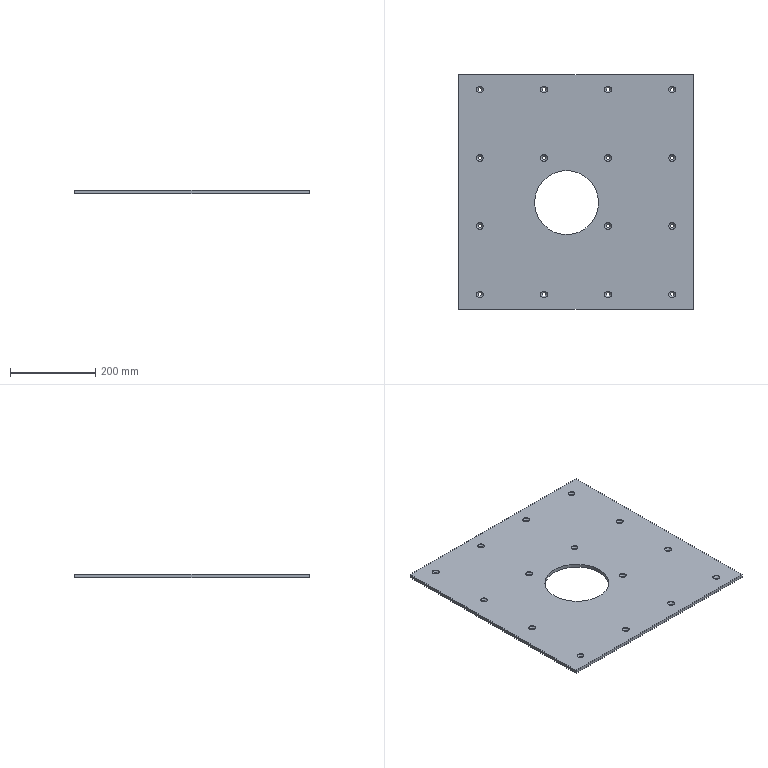Part | STEP file | 车灯-后视镜_id582_x_t | 1 solid | 52 faces | box 550 x 550 x 8 mm | volume 2264649 mm3 | cylinder 31 | cone 15 | plane 6 | commonest cylinder face diameters 8.5 x15 16 x15 150 x1
STEP:
#1=CARTESIAN_POINT('',(275.,-275.,225.5));
#2=VERTEX_POINT('',#1);
#3=CARTESIAN_POINT('',(-275.,-275.,225.5));
#4=VERTEX_POINT('',#3);
#5=CARTESIAN_POINT('',(275.,-275.,225.5));
#6=DIRECTION('',(-1.,0.,0.));
#7=VECTOR('',#6,1.);
#8=LINE('',#5,#7);
#9=EDGE_CURVE('',#2,#4,#8,.T.);
#10=ORIENTED_EDGE('',*,*,#9,.F.);
#11=CARTESIAN_POINT('',(275.,-275.,233.5));
#12=VERTEX_POINT('',#11);
#13=CARTESIAN_POINT('',(275.,-275.,233.5));
#14=DIRECTION('',(0.,0.,-1.));
#15=VECTOR('',#14,1.);
#16=LINE('',#13,#15);
#17=EDGE_CURVE('',#12,#2,#16,.T.);
#18=ORIENTED_EDGE('',*,*,#17,.F.);
#19=CARTESIAN_POINT('',(-275.,-275.,233.5));
#20=VERTEX_POINT('',#19);
#21=CARTESIAN_POINT('',(275.,-275.,233.5));
#22=DIRECTION('',(-1.,0.,0.));
#23=VECTOR('',#22,1.);
#24=LINE('',#21,#23);
#25=EDGE_CURVE('',#12,#20,#24,.T.);
#26=ORIENTED_EDGE('',*,*,#25,.T.);
#27=CARTESIAN_POINT('',(-275.,-275.,233.5));
#28=DIRECTION('',(0.,0.,-1.));
#29=VECTOR('',#28,1.);
#30=LINE('',#27,#29);
#31=EDGE_CURVE('',#20,#4,#30,.T.);
#32=ORIENTED_EDGE('',*,*,#31,.T.);
#33=EDGE_LOOP('',(#10,#18,#26,#32));
#34=FACE_OUTER_BOUND('',#33,.T.);
#35=CARTESIAN_POINT('',(275.,-275.,233.5));
#36=DIRECTION('',(0.,-1.,0.));
#37=DIRECTION('',(0.,0.,-1.));
#38=AXIS2_PLACEMENT_3D('',#35,#36,#37);
#39=PLANE('',#38);
#40=ADVANCED_FACE('',(#34),#39,.T.);
#41=CARTESIAN_POINT('',(-275.,275.,225.5));
#42=VERTEX_POINT('',#41);
#43=CARTESIAN_POINT('',(-275.,-275.,225.5));
#44=DIRECTION('',(0.,1.,0.));
#45=VECTOR('',#44,1.);
#46=LINE('',#43,#45);
#47=EDGE_CURVE('',#4,#42,#46,.T.);
#48=ORIENTED_EDGE('',*,*,#47,.F.);
#49=ORIENTED_EDGE('',*,*,#31,.F.);
#50=CARTESIAN_POINT('',(-275.,275.,233.5));
#51=VERTEX_POINT('',#50);
#52=CARTESIAN_POINT('',(-275.,-275.,233.5));
#53=DIRECTION('',(0.,1.,0.));
#54=VECTOR('',#53,1.);
#55=LINE('',#52,#54);
#56=EDGE_CURVE('',#20,#51,#55,.T.);
#57=ORIENTED_EDGE('',*,*,#56,.T.);
#58=CARTESIAN_POINT('',(-275.,275.,233.5));
#59=DIRECTION('',(0.,0.,-1.));
#60=VECTOR('',#59,1.);
#61=LINE('',#58,#60);
#62=EDGE_CURVE('',#51,#42,#61,.T.);
#63=ORIENTED_EDGE('',*,*,#62,.T.);
#64=EDGE_LOOP('',(#48,#49,#57,#63));
#65=FACE_OUTER_BOUND('',#64,.T.);
#66=CARTESIAN_POINT('',(-275.,-275.,233.5));
#67=DIRECTION('',(-1.,0.,0.));
#68=DIRECTION('',(0.,0.,1.));
#69=AXIS2_PLACEMENT_3D('',#66,#67,#68);
#70=PLANE('',#69);
#71=ADVANCED_FACE('',(#65),#70,.T.);
#72=CARTESIAN_POINT('',(275.,275.,225.5));
#73=VERTEX_POINT('',#72);
#74=CARTESIAN_POINT('',(-275.,275.,225.5));
#75=DIRECTION('',(1.,0.,0.));
#76=VECTOR('',#75,1.);
#77=LINE('',#74,#76);
#78=EDGE_CURVE('',#42,#73,#77,.T.);
#79=ORIENTED_EDGE('',*,*,#78,.F.);
#80=ORIENTED_EDGE('',*,*,#62,.F.);
#81=CARTESIAN_POINT('',(275.,275.,233.5));
#82=VERTEX_POINT('',#81);
#83=CARTESIAN_POINT('',(-275.,275.,233.5));
#84=DIRECTION('',(1.,0.,0.));
#85=VECTOR('',#84,1.);
#86=LINE('',#83,#85);
#87=EDGE_CURVE('',#51,#82,#86,.T.);
#88=ORIENTED_EDGE('',*,*,#87,.T.);
#89=CARTESIAN_POINT('',(275.,275.,233.5));
#90=DIRECTION('',(0.,0.,-1.));
#91=VECTOR('',#90,1.);
#92=LINE('',#89,#91);
#93=EDGE_CURVE('',#82,#73,#92,.T.);
#94=ORIENTED_EDGE('',*,*,#93,.T.);
#95=EDGE_LOOP('',(#79,#80,#88,#94));
#96=FACE_OUTER_BOUND('',#95,.T.);
#97=CARTESIAN_POINT('',(-275.,275.,233.5));
#98=DIRECTION('',(0.,1.,0.));
#99=DIRECTION('',(0.,0.,1.));
#100=AXIS2_PLACEMENT_3D('',#97,#98,#99);
#101=PLANE('',#100);
#102=ADVANCED_FACE('',(#96),#101,.T.);
#103=CARTESIAN_POINT('',(275.,275.,225.5));
#104=DIRECTION('',(0.,-1.,0.));
#105=VECTOR('',#104,1.);
#106=LINE('',#103,#105);
#107=EDGE_CURVE('',#73,#2,#106,.T.);
#108=ORIENTED_EDGE('',*,*,#107,.F.);
#109=ORIENTED_EDGE('',*,*,#93,.F.);
#110=CARTESIAN_POINT('',(275.,275.,233.5));
#111=DIRECTION('',(0.,-1.,0.));
#112=VECTOR('',#111,1.);
#113=LINE('',#110,#112);
#114=EDGE_CURVE('',#82,#12,#113,.T.);
#115=ORIENTED_EDGE('',*,*,#114,.T.);
#116=ORIENTED_EDGE('',*,*,#17,.T.);
#117=EDGE_LOOP('',(#108,#109,#115,#116));
#118=FACE_OUTER_BOUND('',#117,.T.);
#119=CARTESIAN_POINT('',(275.,275.,233.5));
#120=DIRECTION('',(1.,0.,0.));
#121=DIRECTION('',(0.,0.,-1.));
#122=AXIS2_PLACEMENT_3D('',#119,#120,#121);
#123=PLANE('',#122);
#124=ADVANCED_FACE('',(#118),#123,.T.);
#125=CARTESIAN_POINT('',(-233.,240.,233.5));
#126=VERTEX_POINT('',#125);
#127=CARTESIAN_POINT('',(-225.,240.,233.5));
#128=DIRECTION('',(0.,0.,-1.));
#129=DIRECTION('',(-1.,0.,0.));
#130=AXIS2_PLACEMENT_3D('',#127,#128,#129);
#131=CIRCLE('',#130,8.);
#132=EDGE_CURVE('',#126,#126,#131,.T.);
#133=ORIENTED_EDGE('',*,*,#132,.T.);
#134=EDGE_LOOP('',(#133));
#135=FACE_BOUND('',#134,.T.);
#136=CARTESIAN_POINT('',(-233.,-240.,233.5));
#137=VERTEX_POINT('',#136);
#138=CARTESIAN_POINT('',(-225.,-240.,233.5));
#139=DIRECTION('',(0.,0.,-1.));
#140=DIRECTION('',(-1.,0.,0.));
#141=AXIS2_PLACEMENT_3D('',#138,#139,#140);
#142=CIRCLE('',#141,8.);
#143=EDGE_CURVE('',#137,#137,#142,.T.);
#144=ORIENTED_EDGE('',*,*,#143,.T.);
#145=EDGE_LOOP('',(#144));
#146=FACE_BOUND('',#145,.T.);
#147=CARTESIAN_POINT('',(-83.,80.,233.5));
#148=VERTEX_POINT('',#147);
#149=CARTESIAN_POINT('',(-75.,80.,233.5));
#150=DIRECTION('',(0.,0.,-1.));
#151=DIRECTION('',(-1.,0.,0.));
#152=AXIS2_PLACEMENT_3D('',#149,#150,#151);
#153=CIRCLE('',#152,8.);
#154=EDGE_CURVE('',#148,#148,#153,.T.);
#155=ORIENTED_EDGE('',*,*,#154,.T.);
#156=EDGE_LOOP('',(#155));
#157=FACE_BOUND('',#156,.T.);
#158=CARTESIAN_POINT('',(-233.,-80.,233.5));
#159=VERTEX_POINT('',#158);
#160=CARTESIAN_POINT('',(-225.,-80.,233.5));
#161=DIRECTION('',(0.,0.,-1.));
#162=DIRECTION('',(-1.,0.,0.));
#163=AXIS2_PLACEMENT_3D('',#160,#161,#162);
#164=CIRCLE('',#163,8.);
#165=EDGE_CURVE('',#159,#159,#164,.T.);
#166=ORIENTED_EDGE('',*,*,#165,.T.);
#167=EDGE_LOOP('',(#166));
#168=FACE_BOUND('',#167,.T.);
#169=CARTESIAN_POINT('',(-233.,80.,233.5));
#170=VERTEX_POINT('',#169);
#171=CARTESIAN_POINT('',(-225.,80.,233.5));
#172=DIRECTION('',(0.,0.,-1.));
#173=DIRECTION('',(-1.,0.,0.));
#174=AXIS2_PLACEMENT_3D('',#171,#172,#173);
#175=CIRCLE('',#174,8.);
#176=EDGE_CURVE('',#170,#170,#175,.T.);
#177=ORIENTED_EDGE('',*,*,#176,.T.);
#178=EDGE_LOOP('',(#177));
#179=FACE_BOUND('',#178,.T.);
#180=CARTESIAN_POINT('',(-83.,-240.,233.5));
#181=VERTEX_POINT('',#180);
#182=CARTESIAN_POINT('',(-75.,-240.,233.5));
#183=DIRECTION('',(0.,0.,-1.));
#184=DIRECTION('',(-1.,0.,0.));
#185=AXIS2_PLACEMENT_3D('',#182,#183,#184);
#186=CIRCLE('',#185,8.);
#187=EDGE_CURVE('',#181,#181,#186,.T.);
#188=ORIENTED_EDGE('',*,*,#187,.T.);
#189=EDGE_LOOP('',(#188));
#190=FACE_BOUND('',#189,.T.);
#191=CARTESIAN_POINT('',(-83.,240.,233.5));
#192=VERTEX_POINT('',#191);
#193=CARTESIAN_POINT('',(-75.,240.,233.5));
#194=DIRECTION('',(0.,0.,-1.));
#195=DIRECTION('',(-1.,0.,0.));
#196=AXIS2_PLACEMENT_3D('',#193,#194,#195);
#197=CIRCLE('',#196,8.);
#198=EDGE_CURVE('',#192,#192,#197,.T.);
#199=ORIENTED_EDGE('',*,*,#198,.T.);
#200=EDGE_LOOP('',(#199));
#201=FACE_BOUND('',#200,.T.);
#202=CARTESIAN_POINT('',(67.,240.,233.5));
#203=VERTEX_POINT('',#202);
#204=CARTESIAN_POINT('',(75.,240.,233.5));
#205=DIRECTION('',(0.,0.,-1.));
#206=DIRECTION('',(-1.,0.,0.));
#207=AXIS2_PLACEMENT_3D('',#204,#205,#206);
#208=CIRCLE('',#207,8.);
#209=EDGE_CURVE('',#203,#203,#208,.T.);
#210=ORIENTED_EDGE('',*,*,#209,.T.);
#211=EDGE_LOOP('',(#210));
#212=FACE_BOUND('',#211,.T.);
#213=CARTESIAN_POINT('',(217.,80.,233.5));
#214=VERTEX_POINT('',#213);
#215=CARTESIAN_POINT('',(225.,80.,233.5));
#216=DIRECTION('',(0.,0.,-1.));
#217=DIRECTION('',(-1.,0.,0.));
#218=AXIS2_PLACEMENT_3D('',#215,#216,#217);
#219=CIRCLE('',#218,8.);
#220=EDGE_CURVE('',#214,#214,#219,.T.);
#221=ORIENTED_EDGE('',*,*,#220,.T.);
#222=EDGE_LOOP('',(#221));
#223=FACE_BOUND('',#222,.T.);
#224=CARTESIAN_POINT('',(217.,240.,233.5));
#225=VERTEX_POINT('',#224);
#226=CARTESIAN_POINT('',(225.,240.,233.5));
#227=DIRECTION('',(0.,0.,-1.));
#228=DIRECTION('',(-1.,0.,0.));
#229=AXIS2_PLACEMENT_3D('',#226,#227,#228);
#230=CIRCLE('',#229,8.);
#231=EDGE_CURVE('',#225,#225,#230,.T.);
#232=ORIENTED_EDGE('',*,*,#231,.T.);
#233=EDGE_LOOP('',(#232));
#234=FACE_BOUND('',#233,.T.);
#235=CARTESIAN_POINT('',(67.,-240.,233.5));
#236=VERTEX_POINT('',#235);
#237=CARTESIAN_POINT('',(75.,-240.,233.5));
#238=DIRECTION('',(0.,0.,-1.));
#239=DIRECTION('',(-1.,0.,0.));
#240=AXIS2_PLACEMENT_3D('',#237,#238,#239);
#241=CIRCLE('',#240,8.);
#242=EDGE_CURVE('',#236,#236,#241,.T.);
#243=ORIENTED_EDGE('',*,*,#242,.T.);
#244=EDGE_LOOP('',(#243));
#245=FACE_BOUND('',#244,.T.);
#246=CARTESIAN_POINT('',(217.,-240.,233.5));
#247=VERTEX_POINT('',#246);
#248=CARTESIAN_POINT('',(225.,-240.,233.5));
#249=DIRECTION('',(0.,0.,-1.));
#250=DIRECTION('',(-1.,0.,0.));
#251=AXIS2_PLACEMENT_3D('',#248,#249,#250);
#252=CIRCLE('',#251,8.);
#253=EDGE_CURVE('',#247,#247,#252,.T.);
#254=ORIENTED_EDGE('',*,*,#253,.T.);
#255=EDGE_LOOP('',(#254));
#256=FACE_BOUND('',#255,.T.);
#257=CARTESIAN_POINT('',(67.,-80.,233.5));
#258=VERTEX_POINT('',#257);
#259=CARTESIAN_POINT('',(75.,-80.,233.5));
#260=DIRECTION('',(0.,0.,-1.));
#261=DIRECTION('',(-1.,0.,0.));
#262=AXIS2_PLACEMENT_3D('',#259,#260,#261);
#263=CIRCLE('',#262,8.);
#264=EDGE_CURVE('',#258,#258,#263,.T.);
#265=ORIENTED_EDGE('',*,*,#264,.T.);
#266=EDGE_LOOP('',(#265));
#267=FACE_BOUND('',#266,.T.);
#268=CARTESIAN_POINT('',(217.,-80.,233.5));
#269=VERTEX_POINT('',#268);
#270=CARTESIAN_POINT('',(225.,-80.,233.5));
#271=DIRECTION('',(0.,0.,-1.));
#272=DIRECTION('',(-1.,0.,0.));
#273=AXIS2_PLACEMENT_3D('',#270,#271,#272);
#274=CIRCLE('',#273,8.);
#275=EDGE_CURVE('',#269,#269,#274,.T.);
#276=ORIENTED_EDGE('',*,*,#275,.T.);
#277=EDGE_LOOP('',(#276));
#278=FACE_BOUND('',#277,.T.);
#279=CARTESIAN_POINT('',(67.,80.,233.5));
#280=VERTEX_POINT('',#279);
#281=CARTESIAN_POINT('',(75.,80.,233.5));
#282=DIRECTION('',(0.,0.,-1.));
#283=DIRECTION('',(-1.,0.,0.));
#284=AXIS2_PLACEMENT_3D('',#281,#282,#283);
#285=CIRCLE('',#284,8.);
#286=EDGE_CURVE('',#280,#280,#285,.T.);
#287=ORIENTED_EDGE('',*,*,#286,.T.);
#288=EDGE_LOOP('',(#287));
#289=FACE_BOUND('',#288,.T.);
#290=CARTESIAN_POINT('',(-97.,-25.,233.5));
#291=VERTEX_POINT('',#290);
#292=CARTESIAN_POINT('',(-22.,-25.,233.5));
#293=DIRECTION('',(0.,0.,-1.));
#294=DIRECTION('',(-1.,0.,0.));
#295=AXIS2_PLACEMENT_3D('',#292,#293,#294);
#296=CIRCLE('',#295,75.);
#297=EDGE_CURVE('',#291,#291,#296,.T.);
#298=ORIENTED_EDGE('',*,*,#297,.T.);
#299=EDGE_LOOP('',(#298));
#300=FACE_BOUND('',#299,.T.);
#301=ORIENTED_EDGE('',*,*,#25,.F.);
#302=ORIENTED_EDGE('',*,*,#114,.F.);
#303=ORIENTED_EDGE('',*,*,#87,.F.);
#304=ORIENTED_EDGE('',*,*,#56,.F.);
#305=EDGE_LOOP('',(#301,#302,#303,#304));
#306=FACE_BOUND('',#305,.T.);
#307=CARTESIAN_POINT('',(-275.,-275.,233.5));
#308=DIRECTION('',(0.,0.,-1.));
#309=DIRECTION('',(-1.,0.,0.));
#310=AXIS2_PLACEMENT_3D('',#307,#308,#309);
#311=PLANE('',#310);
#312=ADVANCED_FACE('',(#135,#146,#157,#168,#179,#190,#201,#212,#223,#234,#245,#256,#267,#278,#289,#300,#306),#311,.F.);
#313=CARTESIAN_POINT('',(-229.25,240.,225.5));
#314=VERTEX_POINT('',#313);
#315=CARTESIAN_POINT('',(-225.,240.,225.5));
#316=DIRECTION('',(0.,0.,-1.));
#317=DIRECTION('',(-1.,0.,0.));
#318=AXIS2_PLACEMENT_3D('',#315,#316,#317);
#319=CIRCLE('',#318,4.25);
#320=EDGE_CURVE('',#314,#314,#319,.T.);
#321=ORIENTED_EDGE('',*,*,#320,.F.);
#322=EDGE_LOOP('',(#321));
#323=FACE_BOUND('',#322,.T.);
#324=CARTESIAN_POINT('',(-229.25,-240.,225.5));
#325=VERTEX_POINT('',#324);
#326=CARTESIAN_POINT('',(-225.,-240.,225.5));
#327=DIRECTION('',(0.,0.,-1.));
#328=DIRECTION('',(-1.,0.,0.));
#329=AXIS2_PLACEMENT_3D('',#326,#327,#328);
#330=CIRCLE('',#329,4.25);
#331=EDGE_CURVE('',#325,#325,#330,.T.);
#332=ORIENTED_EDGE('',*,*,#331,.F.);
#333=EDGE_LOOP('',(#332));
#334=FACE_BOUND('',#333,.T.);
#335=CARTESIAN_POINT('',(-79.25,80.,225.5));
#336=VERTEX_POINT('',#335);
#337=CARTESIAN_POINT('',(-75.,80.,225.5));
#338=DIRECTION('',(0.,0.,-1.));
#339=DIRECTION('',(-1.,0.,0.));
#340=AXIS2_PLACEMENT_3D('',#337,#338,#339);
#341=CIRCLE('',#340,4.25);
#342=EDGE_CURVE('',#336,#336,#341,.T.);
#343=ORIENTED_EDGE('',*,*,#342,.F.);
#344=EDGE_LOOP('',(#343));
#345=FACE_BOUND('',#344,.T.);
#346=CARTESIAN_POINT('',(-229.25,-80.,225.5));
#347=VERTEX_POINT('',#346);
#348=CARTESIAN_POINT('',(-225.,-80.,225.5));
#349=DIRECTION('',(0.,0.,-1.));
#350=DIRECTION('',(-1.,0.,0.));
#351=AXIS2_PLACEMENT_3D('',#348,#349,#350);
#352=CIRCLE('',#351,4.25);
#353=EDGE_CURVE('',#347,#347,#352,.T.);
#354=ORIENTED_EDGE('',*,*,#353,.F.);
#355=EDGE_LOOP('',(#354));
#356=FACE_BOUND('',#355,.T.);
#357=CARTESIAN_POINT('',(-229.25,80.,225.5));
#358=VERTEX_POINT('',#357);
#359=CARTESIAN_POINT('',(-225.,80.,225.5));
#360=DIRECTION('',(0.,0.,-1.));
#361=DIRECTION('',(-1.,0.,0.));
#362=AXIS2_PLACEMENT_3D('',#359,#360,#361);
#363=CIRCLE('',#362,4.25);
#364=EDGE_CURVE('',#358,#358,#363,.T.);
#365=ORIENTED_EDGE('',*,*,#364,.F.);
#366=EDGE_LOOP('',(#365));
#367=FACE_BOUND('',#366,.T.);
#368=CARTESIAN_POINT('',(-79.25,-240.,225.5));
#369=VERTEX_POINT('',#368);
#370=CARTESIAN_POINT('',(-75.,-240.,225.5));
#371=DIRECTION('',(0.,0.,-1.));
#372=DIRECTION('',(-1.,0.,0.));
#373=AXIS2_PLACEMENT_3D('',#370,#371,#372);
#374=CIRCLE('',#373,4.25);
#375=EDGE_CURVE('',#369,#369,#374,.T.);
#376=ORIENTED_EDGE('',*,*,#375,.F.);
#377=EDGE_LOOP('',(#376));
#378=FACE_BOUND('',#377,.T.);
#379=CARTESIAN_POINT('',(-79.25,240.,225.5));
#380=VERTEX_POINT('',#379);
#381=CARTESIAN_POINT('',(-75.,240.,225.5));
#382=DIRECTION('',(0.,0.,-1.));
#383=DIRECTION('',(-1.,0.,0.));
#384=AXIS2_PLACEMENT_3D('',#381,#382,#383);
#385=CIRCLE('',#384,4.25);
#386=EDGE_CURVE('',#380,#380,#385,.T.);
#387=ORIENTED_EDGE('',*,*,#386,.F.);
#388=EDGE_LOOP('',(#387));
#389=FACE_BOUND('',#388,.T.);
#390=CARTESIAN_POINT('',(70.75,240.,225.5));
#391=VERTEX_POINT('',#390);
#392=CARTESIAN_POINT('',(75.,240.,225.5));
#393=DIRECTION('',(0.,0.,-1.));
#394=DIRECTION('',(-1.,0.,0.));
#395=AXIS2_PLACEMENT_3D('',#392,#393,#394);
#396=CIRCLE('',#395,4.25);
#397=EDGE_CURVE('',#391,#391,#396,.T.);
#398=ORIENTED_EDGE('',*,*,#397,.F.);
#399=EDGE_LOOP('',(#398));
#400=FACE_BOUND('',#399,.T.);
#401=CARTESIAN_POINT('',(220.75,80.,225.5));
#402=VERTEX_POINT('',#401);
#403=CARTESIAN_POINT('',(225.,80.,225.5));
#404=DIRECTION('',(0.,0.,-1.));
#405=DIRECTION('',(-1.,0.,0.));
#406=AXIS2_PLACEMENT_3D('',#403,#404,#405);
#407=CIRCLE('',#406,4.25);
#408=EDGE_CURVE('',#402,#402,#407,.T.);
#409=ORIENTED_EDGE('',*,*,#408,.F.);
#410=EDGE_LOOP('',(#409));
#411=FACE_BOUND('',#410,.T.);
#412=CARTESIAN_POINT('',(220.75,240.,225.5));
#413=VERTEX_POINT('',#412);
#414=CARTESIAN_POINT('',(225.,240.,225.5));
#415=DIRECTION('',(0.,0.,-1.));
#416=DIRECTION('',(-1.,0.,0.));
#417=AXIS2_PLACEMENT_3D('',#414,#415,#416);
#418=CIRCLE('',#417,4.25);
#419=EDGE_CURVE('',#413,#413,#418,.T.);
#420=ORIENTED_EDGE('',*,*,#419,.F.);
#421=EDGE_LOOP('',(#420));
#422=FACE_BOUND('',#421,.T.);
#423=CARTESIAN_POINT('',(70.75,-240.,225.5));
#424=VERTEX_POINT('',#423);
#425=CARTESIAN_POINT('',(75.,-240.,225.5));
#426=DIRECTION('',(0.,0.,-1.));
#427=DIRECTION('',(-1.,0.,0.));
#428=AXIS2_PLACEMENT_3D('',#425,#426,#427);
#429=CIRCLE('',#428,4.25);
#430=EDGE_CURVE('',#424,#424,#429,.T.);
#431=ORIENTED_EDGE('',*,*,#430,.F.);
#432=EDGE_LOOP('',(#431));
#433=FACE_BOUND('',#432,.T.);
#434=CARTESIAN_POINT('',(220.75,-240.,225.5));
#435=VERTEX_POINT('',#434);
#436=CARTESIAN_POINT('',(225.,-240.,225.5));
#437=DIRECTION('',(0.,0.,-1.));
#438=DIRECTION('',(-1.,0.,0.));
#439=AXIS2_PLACEMENT_3D('',#436,#437,#438);
#440=CIRCLE('',#439,4.25);
#441=EDGE_CURVE('',#435,#435,#440,.T.);
#442=ORIENTED_EDGE('',*,*,#441,.F.);
#443=EDGE_LOOP('',(#442));
#444=FACE_BOUND('',#443,.T.);
#445=CARTESIAN_POINT('',(70.75,-80.,225.5));
#446=VERTEX_POINT('',#445);
#447=CARTESIAN_POINT('',(75.,-80.,225.5));
#448=DIRECTION('',(0.,0.,-1.));
#449=DIRECTION('',(-1.,0.,0.));
#450=AXIS2_PLACEMENT_3D('',#447,#448,#449);
#451=CIRCLE('',#450,4.25);
#452=EDGE_CURVE('',#446,#446,#451,.T.);
#453=ORIENTED_EDGE('',*,*,#452,.F.);
#454=EDGE_LOOP('',(#453));
#455=FACE_BOUND('',#454,.T.);
#456=CARTESIAN_POINT('',(220.75,-80.,225.5));
#457=VERTEX_POINT('',#456);
#458=CARTESIAN_POINT('',(225.,-80.,225.5));
#459=DIRECTION('',(0.,0.,-1.));
#460=DIRECTION('',(-1.,0.,0.));
#461=AXIS2_PLACEMENT_3D('',#458,#459,#460);
#462=CIRCLE('',#461,4.25);
#463=EDGE_CURVE('',#457,#457,#462,.T.);
#464=ORIENTED_EDGE('',*,*,#463,.F.);
#465=EDGE_LOOP('',(#464));
#466=FACE_BOUND('',#465,.T.);
#467=CARTESIAN_POINT('',(70.75,80.,225.5));
#468=VERTEX_POINT('',#467);
#469=CARTESIAN_POINT('',(75.,80.,225.5));
#470=DIRECTION('',(0.,0.,-1.));
#471=DIRECTION('',(-1.,0.,0.));
#472=AXIS2_PLACEMENT_3D('',#469,#470,#471);
#473=CIRCLE('',#472,4.25);
#474=EDGE_CURVE('',#468,#468,#473,.T.);
#475=ORIENTED_EDGE('',*,*,#474,.F.);
#476=EDGE_LOOP('',(#475));
#477=FACE_BOUND('',#476,.T.);
#478=CARTESIAN_POINT('',(-97.,-25.,225.5));
#479=VERTEX_POINT('',#478);
#480=CARTESIAN_POINT('',(-22.,-25.,225.5));
#481=DIRECTION('',(0.,0.,-1.));
#482=DIRECTION('',(-1.,0.,0.));
#483=AXIS2_PLACEMENT_3D('',#480,#481,#482);
#484=CIRCLE('',#483,75.);
#485=EDGE_CURVE('',#479,#479,#484,.T.);
#486=ORIENTED_EDGE('',*,*,#485,.F.);
#487=EDGE_LOOP('',(#486));
#488=FACE_BOUND('',#487,.T.);
#489=ORIENTED_EDGE('',*,*,#9,.T.);
#490=ORIENTED_EDGE('',*,*,#47,.T.);
#491=ORIENTED_EDGE('',*,*,#78,.T.);
#492=ORIENTED_EDGE('',*,*,#107,.T.);
#493=EDGE_LOOP('',(#489,#490,#491,#492));
#494=FACE_BOUND('',#493,.T.);
#495=CARTESIAN_POINT('',(-275.,-275.,225.5));
#496=DIRECTION('',(0.,0.,-1.));
#497=DIRECTION('',(-1.,0.,0.));
#498=AXIS2_PLACEMENT_3D('',#495,#496,#497);
#499=PLANE('',#498);
#500=ADVANCED_FACE('',(#323,#334,#345,#356,#367,#378,#389,#400,#411,#422,#433,#444,#455,#466,#477,#488,#494),#499,.T.);
#501=ORIENTED_EDGE('',*,*,#485,.T.);
#502=EDGE_LOOP('',(#501));
#503=FACE_BOUND('',#502,.T.);
#504=ORIENTED_EDGE('',*,*,#297,.F.);
#505=EDGE_LOOP('',(#504));
#506=FACE_BOUND('',#505,.T.);
#507=CARTESIAN_POINT('',(-22.,-25.,225.5));
#508=DIRECTION('',(0.,0.,1.));
#509=DIRECTION('',(1.,0.,0.));
#510=AXIS2_PLACEMENT_3D('',#507,#508,#509);
#511=CYLINDRICAL_SURFACE('',#510,75.);
#512=ADVANCED_FACE('',(#503,#506),#511,.F.);
#513=ORIENTED_EDGE('',*,*,#474,.T.);
#514=EDGE_LOOP('',(#513));
#515=FACE_BOUND('',#514,.T.);
#516=CARTESIAN_POINT('',(70.75,80.,228.122));
#517=VERTEX_POINT('',#516);
#518=CARTESIAN_POINT('',(75.,80.,228.122));
#519=DIRECTION('',(0.,0.,-1.));
#520=DIRECTION('',(-1.,0.,0.));
#521=AXIS2_PLACEMENT_3D('',#518,#519,#520);
#522=CIRCLE('',#521,4.25);
#523=EDGE_CURVE('',#517,#517,#522,.T.);
#524=ORIENTED_EDGE('',*,*,#523,.F.);
#525=EDGE_LOOP('',(#524));
#526=FACE_BOUND('',#525,.T.);
#527=CARTESIAN_POINT('',(75.,80.,228.6));
#528=DIRECTION('',(0.,0.,-1.));
#529=DIRECTION('',(1.,0.,0.));
#530=AXIS2_PLACEMENT_3D('',#527,#528,#529);
#531=CYLINDRICAL_SURFACE('',#530,4.25);
#532=ADVANCED_FACE('',(#515,#526),#531,.F.);
#533=CARTESIAN_POINT('',(67.,80.,231.872));
#534=VERTEX_POINT('',#533);
#535=CARTESIAN_POINT('',(75.,80.,231.872));
#536=DIRECTION('',(0.,0.,-1.));
#537=DIRECTION('',(-1.,0.,0.));
#538=AXIS2_PLACEMENT_3D('',#535,#536,#537);
#539=CIRCLE('',#538,8.);
#540=EDGE_CURVE('',#534,#534,#539,.T.);
#541=ORIENTED_EDGE('',*,*,#540,.T.);
#542=EDGE_LOOP('',(#541));
#543=FACE_BOUND('',#542,.T.);
#544=ORIENTED_EDGE('',*,*,#286,.F.);
#545=EDGE_LOOP('',(#544));
#546=FACE_BOUND('',#545,.T.);
#547=CARTESIAN_POINT('',(75.,80.,233.));
#548=DIRECTION('',(0.,0.,-1.));
#549=DIRECTION('',(1.,0.,0.));
#550=AXIS2_PLACEMENT_3D('',#547,#548,#549);
#551=CYLINDRICAL_SURFACE('',#550,8.);
#552=ADVANCED_FACE('',(#543,#546),#551,.F.);
#553=ORIENTED_EDGE('',*,*,#523,.T.);
#554=EDGE_LOOP('',(#553));
#555=FACE_BOUND('',#554,.T.);
#556=ORIENTED_EDGE('',*,*,#540,.F.);
#557=EDGE_LOOP('',(#556));
#558=FACE_BOUND('',#557,.T.);
#559=CARTESIAN_POINT('',(75.,80.,231.286));
#560=DIRECTION('',(0.,0.,1.));
#561=DIRECTION('',(1.,0.,0.));
#562=AXIS2_PLACEMENT_3D('',#559,#560,#561);
#563=CONICAL_SURFACE('',#562,7.414,45.);
#564=ADVANCED_FACE('',(#555,#558),#563,.F.);
#565=ORIENTED_EDGE('',*,*,#463,.T.);
#566=EDGE_LOOP('',(#565));
#567=FACE_BOUND('',#566,.T.);
#568=CARTESIAN_POINT('',(220.75,-80.,228.122));
#569=VERTEX_POINT('',#568);
#570=CARTESIAN_POINT('',(225.,-80.,228.122));
#571=DIRECTION('',(0.,0.,-1.));
#572=DIRECTION('',(-1.,0.,0.));
#573=AXIS2_PLACEMENT_3D('',#570,#571,#572);
#574=CIRCLE('',#573,4.25);
#575=EDGE_CURVE('',#569,#569,#574,.T.);
#576=ORIENTED_EDGE('',*,*,#575,.F.);
#577=EDGE_LOOP('',(#576));
#578=FACE_BOUND('',#577,.T.);
#579=CARTESIAN_POINT('',(225.,-80.,228.6));
#580=DIRECTION('',(0.,0.,-1.));
#581=DIRECTION('',(1.,0.,0.));
#582=AXIS2_PLACEMENT_3D('',#579,#580,#581);
#583=CYLINDRICAL_SURFACE('',#582,4.25);
#584=ADVANCED_FACE('',(#567,#578),#583,.F.);
#585=CARTESIAN_POINT('',(217.,-80.,231.872));
#586=VERTEX_POINT('',#585);
#587=CARTESIAN_POINT('',(225.,-80.,231.872));
#588=DIRECTION('',(0.,0.,-1.));
#589=DIRECTION('',(-1.,0.,0.));
#590=AXIS2_PLACEMENT_3D('',#587,#588,#589);
#591=CIRCLE('',#590,8.);
#592=EDGE_CURVE('',#586,#586,#591,.T.);
#593=ORIENTED_EDGE('',*,*,#592,.T.);
#594=EDGE_LOOP('',(#593));
#595=FACE_BOUND('',#594,.T.);
#596=ORIENTED_EDGE('',*,*,#275,.F.);
#597=EDGE_LOOP('',(#596));
#598=FACE_BOUND('',#597,.T.);
#599=CARTESIAN_POINT('',(225.,-80.,233.));
#600=DIRECTION('',(0.,0.,-1.));
#601=DIRECTION('',(1.,0.,0.));
#602=AXIS2_PLACEMENT_3D('',#599,#600,#601);
#603=CYLINDRICAL_SURFACE('',#602,8.);
#604=ADVANCED_FACE('',(#595,#598),#603,.F.);
#605=ORIENTED_EDGE('',*,*,#575,.T.);
#606=EDGE_LOOP('',(#605));
#607=FACE_BOUND('',#606,.T.);
#608=ORIENTED_EDGE('',*,*,#592,.F.);
#609=EDGE_LOOP('',(#608));
#610=FACE_BOUND('',#609,.T.);
#611=CARTESIAN_POINT('',(225.,-80.,231.286));
#612=DIRECTION('',(0.,0.,1.));
#613=DIRECTION('',(1.,0.,0.));
#614=AXIS2_PLACEMENT_3D('',#611,#612,#613);
#615=CONICAL_SURFACE('',#614,7.414,45.);
#616=ADVANCED_FACE('',(#607,#610),#615,.F.);
#617=ORIENTED_EDGE('',*,*,#452,.T.);
#618=EDGE_LOOP('',(#617));
#619=FACE_BOUND('',#618,.T.);
#620=CARTESIAN_POINT('',(70.75,-80.,228.122));
#621=VERTEX_POINT('',#620);
#622=CARTESIAN_POINT('',(75.,-80.,228.122));
#623=DIRECTION('',(0.,0.,-1.));
#624=DIRECTION('',(-1.,0.,0.));
#625=AXIS2_PLACEMENT_3D('',#622,#623,#624);
#626=CIRCLE('',#625,4.25);
#627=EDGE_CURVE('',#621,#621,#626,.T.);
#628=ORIENTED_EDGE('',*,*,#627,.F.);
#629=EDGE_LOOP('',(#628));
#630=FACE_BOUND('',#629,.T.);
#631=CARTESIAN_POINT('',(75.,-80.,228.6));
#632=DIRECTION('',(0.,0.,-1.));
#633=DIRECTION('',(1.,0.,0.));
#634=AXIS2_PLACEMENT_3D('',#631,#632,#633);
#635=CYLINDRICAL_SURFACE('',#634,4.25);
#636=ADVANCED_FACE('',(#619,#630),#635,.F.);
#637=CARTESIAN_POINT('',(67.,-80.,231.872));
#638=VERTEX_POINT('',#637);
#639=CARTESIAN_POINT('',(75.,-80.,231.872));
#640=DIRECTION('',(0.,0.,-1.));
#641=DIRECTION('',(-1.,0.,0.));
#642=AXIS2_PLACEMENT_3D('',#639,#640,#641);
#643=CIRCLE('',#642,8.);
#644=EDGE_CURVE('',#638,#638,#643,.T.);
#645=ORIENTED_EDGE('',*,*,#644,.T.);
#646=EDGE_LOOP('',(#645));
#647=FACE_BOUND('',#646,.T.);
#648=ORIENTED_EDGE('',*,*,#264,.F.);
#649=EDGE_LOOP('',(#648));
#650=FACE_BOUND('',#649,.T.);
#651=CARTESIAN_POINT('',(75.,-80.,233.));
#652=DIRECTION('',(0.,0.,-1.));
#653=DIRECTION('',(1.,0.,0.));
#654=AXIS2_PLACEMENT_3D('',#651,#652,#653);
#655=CYLINDRICAL_SURFACE('',#654,8.);
#656=ADVANCED_FACE('',(#647,#650),#655,.F.);
#657=ORIENTED_EDGE('',*,*,#627,.T.);
#658=EDGE_LOOP('',(#657));
#659=FACE_BOUND('',#658,.T.);
#660=ORIENTED_EDGE('',*,*,#644,.F.);
#661=EDGE_LOOP('',(#660));
#662=FACE_BOUND('',#661,.T.);
#663=CARTESIAN_POINT('',(75.,-80.,231.286));
#664=DIRECTION('',(0.,0.,1.));
#665=DIRECTION('',(1.,0.,0.));
#666=AXIS2_PLACEMENT_3D('',#663,#664,#665);
#667=CONICAL_SURFACE('',#666,7.414,45.);
#668=ADVANCED_FACE('',(#659,#662),#667,.F.);
#669=ORIENTED_EDGE('',*,*,#441,.T.);
#670=EDGE_LOOP('',(#669));
#671=FACE_BOUND('',#670,.T.);
#672=CARTESIAN_POINT('',(220.75,-240.,228.122));
#673=VERTEX_POINT('',#672);
#674=CARTESIAN_POINT('',(225.,-240.,228.122));
#675=DIRECTION('',(0.,0.,-1.));
#676=DIRECTION('',(-1.,0.,0.));
#677=AXIS2_PLACEMENT_3D('',#674,#675,#676);
#678=CIRCLE('',#677,4.25);
#679=EDGE_CURVE('',#673,#673,#678,.T.);
#680=ORIENTED_EDGE('',*,*,#679,.F.);
#681=EDGE_LOOP('',(#680));
#682=FACE_BOUND('',#681,.T.);
#683=CARTESIAN_POINT('',(225.,-240.,228.6));
#684=DIRECTION('',(0.,0.,-1.));
#685=DIRECTION('',(1.,0.,0.));
#686=AXIS2_PLACEMENT_3D('',#683,#684,#685);
#687=CYLINDRICAL_SURFACE('',#686,4.25);
#688=ADVANCED_FACE('',(#671,#682),#687,.F.);
#689=CARTESIAN_POINT('',(217.,-240.,231.872));
#690=VERTEX_POINT('',#689);
#691=CARTESIAN_POINT('',(225.,-240.,231.872));
#692=DIRECTION('',(0.,0.,-1.));
#693=DIRECTION('',(-1.,0.,0.));
#694=AXIS2_PLACEMENT_3D('',#691,#692,#693);
#695=CIRCLE('',#694,8.);
#696=EDGE_CURVE('',#690,#690,#695,.T.);
#697=ORIENTED_EDGE('',*,*,#696,.T.);
#698=EDGE_LOOP('',(#697));
#699=FACE_BOUND('',#698,.T.);
#700=ORIENTED_EDGE('',*,*,#253,.F.);
#701=EDGE_LOOP('',(#700));
#702=FACE_BOUND('',#701,.T.);
#703=CARTESIAN_POINT('',(225.,-240.,233.));
#704=DIRECTION('',(0.,0.,-1.));
#705=DIRECTION('',(1.,0.,0.));
#706=AXIS2_PLACEMENT_3D('',#703,#704,#705);
#707=CYLINDRICAL_SURFACE('',#706,8.);
#708=ADVANCED_FACE('',(#699,#702),#707,.F.);
#709=ORIENTED_EDGE('',*,*,#679,.T.);
#710=EDGE_LOOP('',(#709));
#711=FACE_BOUND('',#710,.T.);
#712=ORIENTED_EDGE('',*,*,#696,.F.);
#713=EDGE_LOOP('',(#712));
#714=FACE_BOUND('',#713,.T.);
#715=CARTESIAN_POINT('',(225.,-240.,231.286));
#716=DIRECTION('',(0.,0.,1.));
#717=DIRECTION('',(1.,0.,0.));
#718=AXIS2_PLACEMENT_3D('',#715,#716,#717);
#719=CONICAL_SURFACE('',#718,7.414,45.);
#720=ADVANCED_FACE('',(#711,#714),#719,.F.);
#721=ORIENTED_EDGE('',*,*,#430,.T.);
#722=EDGE_LOOP('',(#721));
#723=FACE_BOUND('',#722,.T.);
#724=CARTESIAN_POINT('',(70.75,-240.,228.122));
#725=VERTEX_POINT('',#724);
#726=CARTESIAN_POINT('',(75.,-240.,228.122));
#727=DIRECTION('',(0.,0.,-1.));
#728=DIRECTION('',(-1.,0.,0.));
#729=AXIS2_PLACEMENT_3D('',#726,#727,#728);
#730=CIRCLE('',#729,4.25);
#731=EDGE_CURVE('',#725,#725,#730,.T.);
#732=ORIENTED_EDGE('',*,*,#731,.F.);
#733=EDGE_LOOP('',(#732));
#734=FACE_BOUND('',#733,.T.);
#735=CARTESIAN_POINT('',(75.,-240.,228.6));
#736=DIRECTION('',(0.,0.,-1.));
#737=DIRECTION('',(1.,0.,0.));
#738=AXIS2_PLACEMENT_3D('',#735,#736,#737);
#739=CYLINDRICAL_SURFACE('',#738,4.25);
#740=ADVANCED_FACE('',(#723,#734),#739,.F.);
#741=CARTESIAN_POINT('',(67.,-240.,231.872));
#742=VERTEX_POINT('',#741);
#743=CARTESIAN_POINT('',(75.,-240.,231.872));
#744=DIRECTION('',(0.,0.,-1.));
#745=DIRECTION('',(-1.,0.,0.));
#746=AXIS2_PLACEMENT_3D('',#743,#744,#745);
#747=CIRCLE('',#746,8.);
#748=EDGE_CURVE('',#742,#742,#747,.T.);
#749=ORIENTED_EDGE('',*,*,#748,.T.);
#750=EDGE_LOOP('',(#749));
#751=FACE_BOUND('',#750,.T.);
#752=ORIENTED_EDGE('',*,*,#242,.F.);
#753=EDGE_LOOP('',(#752));
#754=FACE_BOUND('',#753,.T.);
#755=CARTESIAN_POINT('',(75.,-240.,233.));
#756=DIRECTION('',(0.,0.,-1.));
#757=DIRECTION('',(1.,0.,0.));
#758=AXIS2_PLACEMENT_3D('',#755,#756,#757);
#759=CYLINDRICAL_SURFACE('',#758,8.);
#760=ADVANCED_FACE('',(#751,#754),#759,.F.);
#761=ORIENTED_EDGE('',*,*,#731,.T.);
#762=EDGE_LOOP('',(#761));
#763=FACE_BOUND('',#762,.T.);
#764=ORIENTED_EDGE('',*,*,#748,.F.);
#765=EDGE_LOOP('',(#764));
#766=FACE_BOUND('',#765,.T.);
#767=CARTESIAN_POINT('',(75.,-240.,231.286));
#768=DIRECTION('',(0.,0.,1.));
#769=DIRECTION('',(1.,0.,0.));
#770=AXIS2_PLACEMENT_3D('',#767,#768,#769);
#771=CONICAL_SURFACE('',#770,7.414,45.);
#772=ADVANCED_FACE('',(#763,#766),#771,.F.);
#773=ORIENTED_EDGE('',*,*,#419,.T.);
#774=EDGE_LOOP('',(#773));
#775=FACE_BOUND('',#774,.T.);
#776=CARTESIAN_POINT('',(220.75,240.,228.122));
#777=VERTEX_POINT('',#776);
#778=CARTESIAN_POINT('',(225.,240.,228.122));
#779=DIRECTION('',(0.,0.,-1.));
#780=DIRECTION('',(-1.,0.,0.));
#781=AXIS2_PLACEMENT_3D('',#778,#779,#780);
#782=CIRCLE('',#781,4.25);
#783=EDGE_CURVE('',#777,#777,#782,.T.);
#784=ORIENTED_EDGE('',*,*,#783,.F.);
#785=EDGE_LOOP('',(#784));
#786=FACE_BOUND('',#785,.T.);
#787=CARTESIAN_POINT('',(225.,240.,228.6));
#788=DIRECTION('',(0.,0.,-1.));
#789=DIRECTION('',(1.,0.,0.));
#790=AXIS2_PLACEMENT_3D('',#787,#788,#789);
#791=CYLINDRICAL_SURFACE('',#790,4.25);
#792=ADVANCED_FACE('',(#775,#786),#791,.F.);
#793=CARTESIAN_POINT('',(217.,240.,231.872));
#794=VERTEX_POINT('',#793);
#795=CARTESIAN_POINT('',(225.,240.,231.872));
#796=DIRECTION('',(0.,0.,-1.));
#797=DIRECTION('',(-1.,0.,0.));
#798=AXIS2_PLACEMENT_3D('',#795,#796,#797);
#799=CIRCLE('',#798,8.);
#800=EDGE_CURVE('',#794,#794,#799,.T.);
#801=ORIENTED_EDGE('',*,*,#800,.T.);
#802=EDGE_LOOP('',(#801));
#803=FACE_BOUND('',#802,.T.);
#804=ORIENTED_EDGE('',*,*,#231,.F.);
#805=EDGE_LOOP('',(#804));
#806=FACE_BOUND('',#805,.T.);
#807=CARTESIAN_POINT('',(225.,240.,233.));
#808=DIRECTION('',(0.,0.,-1.));
#809=DIRECTION('',(1.,0.,0.));
#810=AXIS2_PLACEMENT_3D('',#807,#808,#809);
#811=CYLINDRICAL_SURFACE('',#810,8.);
#812=ADVANCED_FACE('',(#803,#806),#811,.F.);
#813=ORIENTED_EDGE('',*,*,#783,.T.);
#814=EDGE_LOOP('',(#813));
#815=FACE_BOUND('',#814,.T.);
#816=ORIENTED_EDGE('',*,*,#800,.F.);
#817=EDGE_LOOP('',(#816));
#818=FACE_BOUND('',#817,.T.);
#819=CARTESIAN_POINT('',(225.,240.,231.286));
#820=DIRECTION('',(0.,0.,1.));
#821=DIRECTION('',(1.,0.,0.));
#822=AXIS2_PLACEMENT_3D('',#819,#820,#821);
#823=CONICAL_SURFACE('',#822,7.414,45.);
#824=ADVANCED_FACE('',(#815,#818),#823,.F.);
#825=ORIENTED_EDGE('',*,*,#408,.T.);
#826=EDGE_LOOP('',(#825));
#827=FACE_BOUND('',#826,.T.);
#828=CARTESIAN_POINT('',(220.75,80.,228.122));
#829=VERTEX_POINT('',#828);
#830=CARTESIAN_POINT('',(225.,80.,228.122));
#831=DIRECTION('',(0.,0.,-1.));
#832=DIRECTION('',(-1.,0.,0.));
#833=AXIS2_PLACEMENT_3D('',#830,#831,#832);
#834=CIRCLE('',#833,4.25);
#835=EDGE_CURVE('',#829,#829,#834,.T.);
#836=ORIENTED_EDGE('',*,*,#835,.F.);
#837=EDGE_LOOP('',(#836));
#838=FACE_BOUND('',#837,.T.);
#839=CARTESIAN_POINT('',(225.,80.,228.6));
#840=DIRECTION('',(0.,0.,-1.));
#841=DIRECTION('',(1.,0.,0.));
#842=AXIS2_PLACEMENT_3D('',#839,#840,#841);
#843=CYLINDRICAL_SURFACE('',#842,4.25);
#844=ADVANCED_FACE('',(#827,#838),#843,.F.);
#845=CARTESIAN_POINT('',(217.,80.,231.872));
#846=VERTEX_POINT('',#845);
#847=CARTESIAN_POINT('',(225.,80.,231.872));
#848=DIRECTION('',(0.,0.,-1.));
#849=DIRECTION('',(-1.,0.,0.));
#850=AXIS2_PLACEMENT_3D('',#847,#848,#849);
#851=CIRCLE('',#850,8.);
#852=EDGE_CURVE('',#846,#846,#851,.T.);
#853=ORIENTED_EDGE('',*,*,#852,.T.);
#854=EDGE_LOOP('',(#853));
#855=FACE_BOUND('',#854,.T.);
#856=ORIENTED_EDGE('',*,*,#220,.F.);
#857=EDGE_LOOP('',(#856));
#858=FACE_BOUND('',#857,.T.);
#859=CARTESIAN_POINT('',(225.,80.,233.));
#860=DIRECTION('',(0.,0.,-1.));
#861=DIRECTION('',(1.,0.,0.));
#862=AXIS2_PLACEMENT_3D('',#859,#860,#861);
#863=CYLINDRICAL_SURFACE('',#862,8.);
#864=ADVANCED_FACE('',(#855,#858),#863,.F.);
#865=ORIENTED_EDGE('',*,*,#835,.T.);
#866=EDGE_LOOP('',(#865));
#867=FACE_BOUND('',#866,.T.);
#868=ORIENTED_EDGE('',*,*,#852,.F.);
#869=EDGE_LOOP('',(#868));
#870=FACE_BOUND('',#869,.T.);
#871=CARTESIAN_POINT('',(225.,80.,231.286));
#872=DIRECTION('',(0.,0.,1.));
#873=DIRECTION('',(1.,0.,0.));
#874=AXIS2_PLACEMENT_3D('',#871,#872,#873);
#875=CONICAL_SURFACE('',#874,7.414,45.);
#876=ADVANCED_FACE('',(#867,#870),#875,.F.);
#877=ORIENTED_EDGE('',*,*,#397,.T.);
#878=EDGE_LOOP('',(#877));
#879=FACE_BOUND('',#878,.T.);
#880=CARTESIAN_POINT('',(70.75,240.,228.122));
#881=VERTEX_POINT('',#880);
#882=CARTESIAN_POINT('',(75.,240.,228.122));
#883=DIRECTION('',(0.,0.,-1.));
#884=DIRECTION('',(-1.,0.,0.));
#885=AXIS2_PLACEMENT_3D('',#882,#883,#884);
#886=CIRCLE('',#885,4.25);
#887=EDGE_CURVE('',#881,#881,#886,.T.);
#888=ORIENTED_EDGE('',*,*,#887,.F.);
#889=EDGE_LOOP('',(#888));
#890=FACE_BOUND('',#889,.T.);
#891=CARTESIAN_POINT('',(75.,240.,228.6));
#892=DIRECTION('',(0.,0.,-1.));
#893=DIRECTION('',(1.,0.,0.));
#894=AXIS2_PLACEMENT_3D('',#891,#892,#893);
#895=CYLINDRICAL_SURFACE('',#894,4.25);
#896=ADVANCED_FACE('',(#879,#890),#895,.F.);
#897=CARTESIAN_POINT('',(67.,240.,231.872));
#898=VERTEX_POINT('',#897);
#899=CARTESIAN_POINT('',(75.,240.,231.872));
#900=DIRECTION('',(0.,0.,-1.));
#901=DIRECTION('',(-1.,0.,0.));
#902=AXIS2_PLACEMENT_3D('',#899,#900,#901);
#903=CIRCLE('',#902,8.);
#904=EDGE_CURVE('',#898,#898,#903,.T.);
#905=ORIENTED_EDGE('',*,*,#904,.T.);
#906=EDGE_LOOP('',(#905));
#907=FACE_BOUND('',#906,.T.);
#908=ORIENTED_EDGE('',*,*,#209,.F.);
#909=EDGE_LOOP('',(#908));
#910=FACE_BOUND('',#909,.T.);
#911=CARTESIAN_POINT('',(75.,240.,233.));
#912=DIRECTION('',(0.,0.,-1.));
#913=DIRECTION('',(1.,0.,0.));
#914=AXIS2_PLACEMENT_3D('',#911,#912,#913);
#915=CYLINDRICAL_SURFACE('',#914,8.);
#916=ADVANCED_FACE('',(#907,#910),#915,.F.);
#917=ORIENTED_EDGE('',*,*,#887,.T.);
#918=EDGE_LOOP('',(#917));
#919=FACE_BOUND('',#918,.T.);
#920=ORIENTED_EDGE('',*,*,#904,.F.);
#921=EDGE_LOOP('',(#920));
#922=FACE_BOUND('',#921,.T.);
#923=CARTESIAN_POINT('',(75.,240.,231.286));
#924=DIRECTION('',(0.,0.,1.));
#925=DIRECTION('',(1.,0.,0.));
#926=AXIS2_PLACEMENT_3D('',#923,#924,#925);
#927=CONICAL_SURFACE('',#926,7.414,45.);
#928=ADVANCED_FACE('',(#919,#922),#927,.F.);
#929=ORIENTED_EDGE('',*,*,#386,.T.);
#930=EDGE_LOOP('',(#929));
#931=FACE_BOUND('',#930,.T.);
#932=CARTESIAN_POINT('',(-79.25,240.,228.122));
#933=VERTEX_POINT('',#932);
#934=CARTESIAN_POINT('',(-75.,240.,228.122));
#935=DIRECTION('',(0.,0.,-1.));
#936=DIRECTION('',(-1.,0.,0.));
#937=AXIS2_PLACEMENT_3D('',#934,#935,#936);
#938=CIRCLE('',#937,4.25);
#939=EDGE_CURVE('',#933,#933,#938,.T.);
#940=ORIENTED_EDGE('',*,*,#939,.F.);
#941=EDGE_LOOP('',(#940));
#942=FACE_BOUND('',#941,.T.);
#943=CARTESIAN_POINT('',(-75.,240.,228.6));
#944=DIRECTION('',(0.,0.,-1.));
#945=DIRECTION('',(1.,0.,0.));
#946=AXIS2_PLACEMENT_3D('',#943,#944,#945);
#947=CYLINDRICAL_SURFACE('',#946,4.25);
#948=ADVANCED_FACE('',(#931,#942),#947,.F.);
#949=CARTESIAN_POINT('',(-83.,240.,231.872));
#950=VERTEX_POINT('',#949);
#951=CARTESIAN_POINT('',(-75.,240.,231.872));
#952=DIRECTION('',(0.,0.,-1.));
#953=DIRECTION('',(-1.,0.,0.));
#954=AXIS2_PLACEMENT_3D('',#951,#952,#953);
#955=CIRCLE('',#954,8.);
#956=EDGE_CURVE('',#950,#950,#955,.T.);
#957=ORIENTED_EDGE('',*,*,#956,.T.);
#958=EDGE_LOOP('',(#957));
#959=FACE_BOUND('',#958,.T.);
#960=ORIENTED_EDGE('',*,*,#198,.F.);
#961=EDGE_LOOP('',(#960));
#962=FACE_BOUND('',#961,.T.);
#963=CARTESIAN_POINT('',(-75.,240.,233.));
#964=DIRECTION('',(0.,0.,-1.));
#965=DIRECTION('',(1.,0.,0.));
#966=AXIS2_PLACEMENT_3D('',#963,#964,#965);
#967=CYLINDRICAL_SURFACE('',#966,8.);
#968=ADVANCED_FACE('',(#959,#962),#967,.F.);
#969=ORIENTED_EDGE('',*,*,#939,.T.);
#970=EDGE_LOOP('',(#969));
#971=FACE_BOUND('',#970,.T.);
#972=ORIENTED_EDGE('',*,*,#956,.F.);
#973=EDGE_LOOP('',(#972));
#974=FACE_BOUND('',#973,.T.);
#975=CARTESIAN_POINT('',(-75.,240.,231.286));
#976=DIRECTION('',(0.,0.,1.));
#977=DIRECTION('',(1.,0.,0.));
#978=AXIS2_PLACEMENT_3D('',#975,#976,#977);
#979=CONICAL_SURFACE('',#978,7.414,45.);
#980=ADVANCED_FACE('',(#971,#974),#979,.F.);
#981=ORIENTED_EDGE('',*,*,#375,.T.);
#982=EDGE_LOOP('',(#981));
#983=FACE_BOUND('',#982,.T.);
#984=CARTESIAN_POINT('',(-79.25,-240.,228.122));
#985=VERTEX_POINT('',#984);
#986=CARTESIAN_POINT('',(-75.,-240.,228.122));
#987=DIRECTION('',(0.,0.,-1.));
#988=DIRECTION('',(-1.,0.,0.));
#989=AXIS2_PLACEMENT_3D('',#986,#987,#988);
#990=CIRCLE('',#989,4.25);
#991=EDGE_CURVE('',#985,#985,#990,.T.);
#992=ORIENTED_EDGE('',*,*,#991,.F.);
#993=EDGE_LOOP('',(#992));
#994=FACE_BOUND('',#993,.T.);
#995=CARTESIAN_POINT('',(-75.,-240.,228.6));
#996=DIRECTION('',(0.,0.,-1.));
#997=DIRECTION('',(1.,0.,0.));
#998=AXIS2_PLACEMENT_3D('',#995,#996,#997);
#999=CYLINDRICAL_SURFACE('',#998,4.25);
#1000=ADVANCED_FACE('',(#983,#994),#999,.F.);
#1001=CARTESIAN_POINT('',(-83.,-240.,231.872));
#1002=VERTEX_POINT('',#1001);
#1003=CARTESIAN_POINT('',(-75.,-240.,231.872));
#1004=DIRECTION('',(0.,0.,-1.));
#1005=DIRECTION('',(-1.,0.,0.));
#1006=AXIS2_PLACEMENT_3D('',#1003,#1004,#1005);
#1007=CIRCLE('',#1006,8.);
#1008=EDGE_CURVE('',#1002,#1002,#1007,.T.);
#1009=ORIENTED_EDGE('',*,*,#1008,.T.);
#1010=EDGE_LOOP('',(#1009));
#1011=FACE_BOUND('',#1010,.T.);
#1012=ORIENTED_EDGE('',*,*,#187,.F.);
#1013=EDGE_LOOP('',(#1012));
#1014=FACE_BOUND('',#1013,.T.);
#1015=CARTESIAN_POINT('',(-75.,-240.,233.));
#1016=DIRECTION('',(0.,0.,-1.));
#1017=DIRECTION('',(1.,0.,0.));
#1018=AXIS2_PLACEMENT_3D('',#1015,#1016,#1017);
#1019=CYLINDRICAL_SURFACE('',#1018,8.);
#1020=ADVANCED_FACE('',(#1011,#1014),#1019,.F.);
#1021=ORIENTED_EDGE('',*,*,#991,.T.);
#1022=EDGE_LOOP('',(#1021));
#1023=FACE_BOUND('',#1022,.T.);
#1024=ORIENTED_EDGE('',*,*,#1008,.F.);
#1025=EDGE_LOOP('',(#1024));
#1026=FACE_BOUND('',#1025,.T.);
#1027=CARTESIAN_POINT('',(-75.,-240.,231.286));
#1028=DIRECTION('',(0.,0.,1.));
#1029=DIRECTION('',(1.,0.,0.));
#1030=AXIS2_PLACEMENT_3D('',#1027,#1028,#1029);
#1031=CONICAL_SURFACE('',#1030,7.414,45.);
#1032=ADVANCED_FACE('',(#1023,#1026),#1031,.F.);
#1033=ORIENTED_EDGE('',*,*,#364,.T.);
#1034=EDGE_LOOP('',(#1033));
#1035=FACE_BOUND('',#1034,.T.);
#1036=CARTESIAN_POINT('',(-229.25,80.,228.122));
#1037=VERTEX_POINT('',#1036);
#1038=CARTESIAN_POINT('',(-225.,80.,228.122));
#1039=DIRECTION('',(0.,0.,-1.));
#1040=DIRECTION('',(-1.,0.,0.));
#1041=AXIS2_PLACEMENT_3D('',#1038,#1039,#1040);
#1042=CIRCLE('',#1041,4.25);
#1043=EDGE_CURVE('',#1037,#1037,#1042,.T.);
#1044=ORIENTED_EDGE('',*,*,#1043,.F.);
#1045=EDGE_LOOP('',(#1044));
#1046=FACE_BOUND('',#1045,.T.);
#1047=CARTESIAN_POINT('',(-225.,80.,228.6));
#1048=DIRECTION('',(0.,0.,-1.));
#1049=DIRECTION('',(1.,0.,0.));
#1050=AXIS2_PLACEMENT_3D('',#1047,#1048,#1049);
#1051=CYLINDRICAL_SURFACE('',#1050,4.25);
#1052=ADVANCED_FACE('',(#1035,#1046),#1051,.F.);
#1053=CARTESIAN_POINT('',(-233.,80.,231.872));
#1054=VERTEX_POINT('',#1053);
#1055=CARTESIAN_POINT('',(-225.,80.,231.872));
#1056=DIRECTION('',(0.,0.,-1.));
#1057=DIRECTION('',(-1.,0.,0.));
#1058=AXIS2_PLACEMENT_3D('',#1055,#1056,#1057);
#1059=CIRCLE('',#1058,8.);
#1060=EDGE_CURVE('',#1054,#1054,#1059,.T.);
#1061=ORIENTED_EDGE('',*,*,#1060,.T.);
#1062=EDGE_LOOP('',(#1061));
#1063=FACE_BOUND('',#1062,.T.);
#1064=ORIENTED_EDGE('',*,*,#176,.F.);
#1065=EDGE_LOOP('',(#1064));
#1066=FACE_BOUND('',#1065,.T.);
#1067=CARTESIAN_POINT('',(-225.,80.,233.));
#1068=DIRECTION('',(0.,0.,-1.));
#1069=DIRECTION('',(1.,0.,0.));
#1070=AXIS2_PLACEMENT_3D('',#1067,#1068,#1069);
#1071=CYLINDRICAL_SURFACE('',#1070,8.);
#1072=ADVANCED_FACE('',(#1063,#1066),#1071,.F.);
#1073=ORIENTED_EDGE('',*,*,#1043,.T.);
#1074=EDGE_LOOP('',(#1073));
#1075=FACE_BOUND('',#1074,.T.);
#1076=ORIENTED_EDGE('',*,*,#1060,.F.);
#1077=EDGE_LOOP('',(#1076));
#1078=FACE_BOUND('',#1077,.T.);
#1079=CARTESIAN_POINT('',(-225.,80.,231.286));
#1080=DIRECTION('',(0.,0.,1.));
#1081=DIRECTION('',(1.,0.,0.));
#1082=AXIS2_PLACEMENT_3D('',#1079,#1080,#1081);
#1083=CONICAL_SURFACE('',#1082,7.414,45.);
#1084=ADVANCED_FACE('',(#1075,#1078),#1083,.F.);
#1085=ORIENTED_EDGE('',*,*,#353,.T.);
#1086=EDGE_LOOP('',(#1085));
#1087=FACE_BOUND('',#1086,.T.);
#1088=CARTESIAN_POINT('',(-229.25,-80.,228.122));
#1089=VERTEX_POINT('',#1088);
#1090=CARTESIAN_POINT('',(-225.,-80.,228.122));
#1091=DIRECTION('',(0.,0.,-1.));
#1092=DIRECTION('',(-1.,0.,0.));
#1093=AXIS2_PLACEMENT_3D('',#1090,#1091,#1092);
#1094=CIRCLE('',#1093,4.25);
#1095=EDGE_CURVE('',#1089,#1089,#1094,.T.);
#1096=ORIENTED_EDGE('',*,*,#1095,.F.);
#1097=EDGE_LOOP('',(#1096));
#1098=FACE_BOUND('',#1097,.T.);
#1099=CARTESIAN_POINT('',(-225.,-80.,228.6));
#1100=DIRECTION('',(0.,0.,-1.));
#1101=DIRECTION('',(1.,0.,0.));
#1102=AXIS2_PLACEMENT_3D('',#1099,#1100,#1101);
#1103=CYLINDRICAL_SURFACE('',#1102,4.25);
#1104=ADVANCED_FACE('',(#1087,#1098),#1103,.F.);
#1105=CARTESIAN_POINT('',(-233.,-80.,231.872));
#1106=VERTEX_POINT('',#1105);
#1107=CARTESIAN_POINT('',(-225.,-80.,231.872));
#1108=DIRECTION('',(0.,0.,-1.));
#1109=DIRECTION('',(-1.,0.,0.));
#1110=AXIS2_PLACEMENT_3D('',#1107,#1108,#1109);
#1111=CIRCLE('',#1110,8.);
#1112=EDGE_CURVE('',#1106,#1106,#1111,.T.);
#1113=ORIENTED_EDGE('',*,*,#1112,.T.);
#1114=EDGE_LOOP('',(#1113));
#1115=FACE_BOUND('',#1114,.T.);
#1116=ORIENTED_EDGE('',*,*,#165,.F.);
#1117=EDGE_LOOP('',(#1116));
#1118=FACE_BOUND('',#1117,.T.);
#1119=CARTESIAN_POINT('',(-225.,-80.,233.));
#1120=DIRECTION('',(0.,0.,-1.));
#1121=DIRECTION('',(1.,0.,0.));
#1122=AXIS2_PLACEMENT_3D('',#1119,#1120,#1121);
#1123=CYLINDRICAL_SURFACE('',#1122,8.);
#1124=ADVANCED_FACE('',(#1115,#1118),#1123,.F.);
#1125=ORIENTED_EDGE('',*,*,#1095,.T.);
#1126=EDGE_LOOP('',(#1125));
#1127=FACE_BOUND('',#1126,.T.);
#1128=ORIENTED_EDGE('',*,*,#1112,.F.);
#1129=EDGE_LOOP('',(#1128));
#1130=FACE_BOUND('',#1129,.T.);
#1131=CARTESIAN_POINT('',(-225.,-80.,231.286));
#1132=DIRECTION('',(0.,0.,1.));
#1133=DIRECTION('',(1.,0.,0.));
#1134=AXIS2_PLACEMENT_3D('',#1131,#1132,#1133);
#1135=CONICAL_SURFACE('',#1134,7.414,45.);
#1136=ADVANCED_FACE('',(#1127,#1130),#1135,.F.);
#1137=ORIENTED_EDGE('',*,*,#342,.T.);
#1138=EDGE_LOOP('',(#1137));
#1139=FACE_BOUND('',#1138,.T.);
#1140=CARTESIAN_POINT('',(-79.25,80.,228.122));
#1141=VERTEX_POINT('',#1140);
#1142=CARTESIAN_POINT('',(-75.,80.,228.122));
#1143=DIRECTION('',(0.,0.,-1.));
#1144=DIRECTION('',(-1.,0.,0.));
#1145=AXIS2_PLACEMENT_3D('',#1142,#1143,#1144);
#1146=CIRCLE('',#1145,4.25);
#1147=EDGE_CURVE('',#1141,#1141,#1146,.T.);
#1148=ORIENTED_EDGE('',*,*,#1147,.F.);
#1149=EDGE_LOOP('',(#1148));
#1150=FACE_BOUND('',#1149,.T.);
#1151=CARTESIAN_POINT('',(-75.,80.,228.6));
#1152=DIRECTION('',(0.,0.,-1.));
#1153=DIRECTION('',(1.,0.,0.));
#1154=AXIS2_PLACEMENT_3D('',#1151,#1152,#1153);
#1155=CYLINDRICAL_SURFACE('',#1154,4.25);
#1156=ADVANCED_FACE('',(#1139,#1150),#1155,.F.);
#1157=CARTESIAN_POINT('',(-83.,80.,231.872));
#1158=VERTEX_POINT('',#1157);
#1159=CARTESIAN_POINT('',(-75.,80.,231.872));
#1160=DIRECTION('',(0.,0.,-1.));
#1161=DIRECTION('',(-1.,0.,0.));
#1162=AXIS2_PLACEMENT_3D('',#1159,#1160,#1161);
#1163=CIRCLE('',#1162,8.);
#1164=EDGE_CURVE('',#1158,#1158,#1163,.T.);
#1165=ORIENTED_EDGE('',*,*,#1164,.T.);
#1166=EDGE_LOOP('',(#1165));
#1167=FACE_BOUND('',#1166,.T.);
#1168=ORIENTED_EDGE('',*,*,#154,.F.);
#1169=EDGE_LOOP('',(#1168));
#1170=FACE_BOUND('',#1169,.T.);
#1171=CARTESIAN_POINT('',(-75.,80.,233.));
#1172=DIRECTION('',(0.,0.,-1.));
#1173=DIRECTION('',(1.,0.,0.));
#1174=AXIS2_PLACEMENT_3D('',#1171,#1172,#1173);
#1175=CYLINDRICAL_SURFACE('',#1174,8.);
#1176=ADVANCED_FACE('',(#1167,#1170),#1175,.F.);
#1177=ORIENTED_EDGE('',*,*,#1147,.T.);
#1178=EDGE_LOOP('',(#1177));
#1179=FACE_BOUND('',#1178,.T.);
#1180=ORIENTED_EDGE('',*,*,#1164,.F.);
#1181=EDGE_LOOP('',(#1180));
#1182=FACE_BOUND('',#1181,.T.);
#1183=CARTESIAN_POINT('',(-75.,80.,231.286));
#1184=DIRECTION('',(0.,0.,1.));
#1185=DIRECTION('',(1.,0.,0.));
#1186=AXIS2_PLACEMENT_3D('',#1183,#1184,#1185);
#1187=CONICAL_SURFACE('',#1186,7.414,45.);
#1188=ADVANCED_FACE('',(#1179,#1182),#1187,.F.);
#1189=ORIENTED_EDGE('',*,*,#331,.T.);
#1190=EDGE_LOOP('',(#1189));
#1191=FACE_BOUND('',#1190,.T.);
#1192=CARTESIAN_POINT('',(-229.25,-240.,228.122));
#1193=VERTEX_POINT('',#1192);
#1194=CARTESIAN_POINT('',(-225.,-240.,228.122));
#1195=DIRECTION('',(0.,0.,-1.));
#1196=DIRECTION('',(-1.,0.,0.));
#1197=AXIS2_PLACEMENT_3D('',#1194,#1195,#1196);
#1198=CIRCLE('',#1197,4.25);
#1199=EDGE_CURVE('',#1193,#1193,#1198,.T.);
#1200=ORIENTED_EDGE('',*,*,#1199,.F.);
#1201=EDGE_LOOP('',(#1200));
#1202=FACE_BOUND('',#1201,.T.);
#1203=CARTESIAN_POINT('',(-225.,-240.,228.6));
#1204=DIRECTION('',(0.,0.,-1.));
#1205=DIRECTION('',(1.,0.,0.));
#1206=AXIS2_PLACEMENT_3D('',#1203,#1204,#1205);
#1207=CYLINDRICAL_SURFACE('',#1206,4.25);
#1208=ADVANCED_FACE('',(#1191,#1202),#1207,.F.);
#1209=CARTESIAN_POINT('',(-233.,-240.,231.872));
#1210=VERTEX_POINT('',#1209);
#1211=CARTESIAN_POINT('',(-225.,-240.,231.872));
#1212=DIRECTION('',(0.,0.,-1.));
#1213=DIRECTION('',(-1.,0.,0.));
#1214=AXIS2_PLACEMENT_3D('',#1211,#1212,#1213);
#1215=CIRCLE('',#1214,8.);
#1216=EDGE_CURVE('',#1210,#1210,#1215,.T.);
#1217=ORIENTED_EDGE('',*,*,#1216,.T.);
#1218=EDGE_LOOP('',(#1217));
#1219=FACE_BOUND('',#1218,.T.);
#1220=ORIENTED_EDGE('',*,*,#143,.F.);
#1221=EDGE_LOOP('',(#1220));
#1222=FACE_BOUND('',#1221,.T.);
#1223=CARTESIAN_POINT('',(-225.,-240.,233.));
#1224=DIRECTION('',(0.,0.,-1.));
#1225=DIRECTION('',(1.,0.,0.));
#1226=AXIS2_PLACEMENT_3D('',#1223,#1224,#1225);
#1227=CYLINDRICAL_SURFACE('',#1226,8.);
#1228=ADVANCED_FACE('',(#1219,#1222),#1227,.F.);
#1229=ORIENTED_EDGE('',*,*,#1199,.T.);
#1230=EDGE_LOOP('',(#1229));
#1231=FACE_BOUND('',#1230,.T.);
#1232=ORIENTED_EDGE('',*,*,#1216,.F.);
#1233=EDGE_LOOP('',(#1232));
#1234=FACE_BOUND('',#1233,.T.);
#1235=CARTESIAN_POINT('',(-225.,-240.,231.286));
#1236=DIRECTION('',(0.,0.,1.));
#1237=DIRECTION('',(1.,0.,0.));
#1238=AXIS2_PLACEMENT_3D('',#1235,#1236,#1237);
#1239=CONICAL_SURFACE('',#1238,7.414,45.);
#1240=ADVANCED_FACE('',(#1231,#1234),#1239,.F.);
#1241=ORIENTED_EDGE('',*,*,#320,.T.);
#1242=EDGE_LOOP('',(#1241));
#1243=FACE_BOUND('',#1242,.T.);
#1244=CARTESIAN_POINT('',(-229.25,240.,228.122));
#1245=VERTEX_POINT('',#1244);
#1246=CARTESIAN_POINT('',(-225.,240.,228.122));
#1247=DIRECTION('',(0.,0.,-1.));
#1248=DIRECTION('',(-1.,0.,0.));
#1249=AXIS2_PLACEMENT_3D('',#1246,#1247,#1248);
#1250=CIRCLE('',#1249,4.25);
#1251=EDGE_CURVE('',#1245,#1245,#1250,.T.);
#1252=ORIENTED_EDGE('',*,*,#1251,.F.);
#1253=EDGE_LOOP('',(#1252));
#1254=FACE_BOUND('',#1253,.T.);
#1255=CARTESIAN_POINT('',(-225.,240.,228.6));
#1256=DIRECTION('',(0.,0.,-1.));
#1257=DIRECTION('',(1.,0.,0.));
#1258=AXIS2_PLACEMENT_3D('',#1255,#1256,#1257);
#1259=CYLINDRICAL_SURFACE('',#1258,4.25);
#1260=ADVANCED_FACE('',(#1243,#1254),#1259,.F.);
#1261=CARTESIAN_POINT('',(-233.,240.,231.872));
#1262=VERTEX_POINT('',#1261);
#1263=CARTESIAN_POINT('',(-225.,240.,231.872));
#1264=DIRECTION('',(0.,0.,-1.));
#1265=DIRECTION('',(-1.,0.,0.));
#1266=AXIS2_PLACEMENT_3D('',#1263,#1264,#1265);
#1267=CIRCLE('',#1266,8.);
#1268=EDGE_CURVE('',#1262,#1262,#1267,.T.);
#1269=ORIENTED_EDGE('',*,*,#1268,.T.);
#1270=EDGE_LOOP('',(#1269));
#1271=FACE_BOUND('',#1270,.T.);
#1272=ORIENTED_EDGE('',*,*,#132,.F.);
#1273=EDGE_LOOP('',(#1272));
#1274=FACE_BOUND('',#1273,.T.);
#1275=CARTESIAN_POINT('',(-225.,240.,233.));
#1276=DIRECTION('',(0.,0.,-1.));
#1277=DIRECTION('',(1.,0.,0.));
#1278=AXIS2_PLACEMENT_3D('',#1275,#1276,#1277);
#1279=CYLINDRICAL_SURFACE('',#1278,8.);
#1280=ADVANCED_FACE('',(#1271,#1274),#1279,.F.);
#1281=ORIENTED_EDGE('',*,*,#1251,.T.);
#1282=EDGE_LOOP('',(#1281));
#1283=FACE_BOUND('',#1282,.T.);
#1284=ORIENTED_EDGE('',*,*,#1268,.F.);
#1285=EDGE_LOOP('',(#1284));
#1286=FACE_BOUND('',#1285,.T.);
#1287=CARTESIAN_POINT('',(-225.,240.,231.286));
#1288=DIRECTION('',(0.,0.,1.));
#1289=DIRECTION('',(1.,0.,0.));
#1290=AXIS2_PLACEMENT_3D('',#1287,#1288,#1289);
#1291=CONICAL_SURFACE('',#1290,7.414,45.);
#1292=ADVANCED_FACE('',(#1283,#1286),#1291,.F.);
#1293=CLOSED_SHELL('',(#40,#71,#102,#124,#312,#500,#512,#532,#552,#564,#584,#604,#616,#636,#656,#668,#688,#708,#720,#740,#760,#772,#792,#812,#824,#844,#864,#876,#896,#916,#928,#948,#968,#980,#1000,#1020,#1032,#1052,#1072,#1084,#1104,#1124,#1136,#1156,#1176,#1188,#1208,#1228,#1240,#1260,#1280,#1292));
#1294=MANIFOLD_SOLID_BREP('',#1293);
#1295=(LENGTH_UNIT()NAMED_UNIT(*)SI_UNIT(.MILLI.,.METRE.));
#1296=UNCERTAINTY_MEASURE_WITH_UNIT(LENGTH_MEASURE(0.00002),#1295,'','');
#1297=(NAMED_UNIT(*)PLANE_ANGLE_UNIT()SI_UNIT($,.RADIAN.));
#1298=PLANE_ANGLE_MEASURE_WITH_UNIT(PLANE_ANGLE_MEASURE(0.01745),#1297);
#1299=DIMENSIONAL_EXPONENTS(0.,0.,0.,0.,0.,0.,0.);
#1300=(CONVERSION_BASED_UNIT('DEGREE',#1298)NAMED_UNIT(#1299)PLANE_ANGLE_UNIT());
#1301=(NAMED_UNIT(*)SI_UNIT($,.STERADIAN.)SOLID_ANGLE_UNIT());
#1302=(GEOMETRIC_REPRESENTATION_CONTEXT(3)GLOBAL_UNCERTAINTY_ASSIGNED_CONTEXT((#1296))GLOBAL_UNIT_ASSIGNED_CONTEXT((#1295,#1300,#1301))REPRESENTATION_CONTEXT('',''));
#1303=ADVANCED_BREP_SHAPE_REPRESENTATION('',(#1294),#1302);